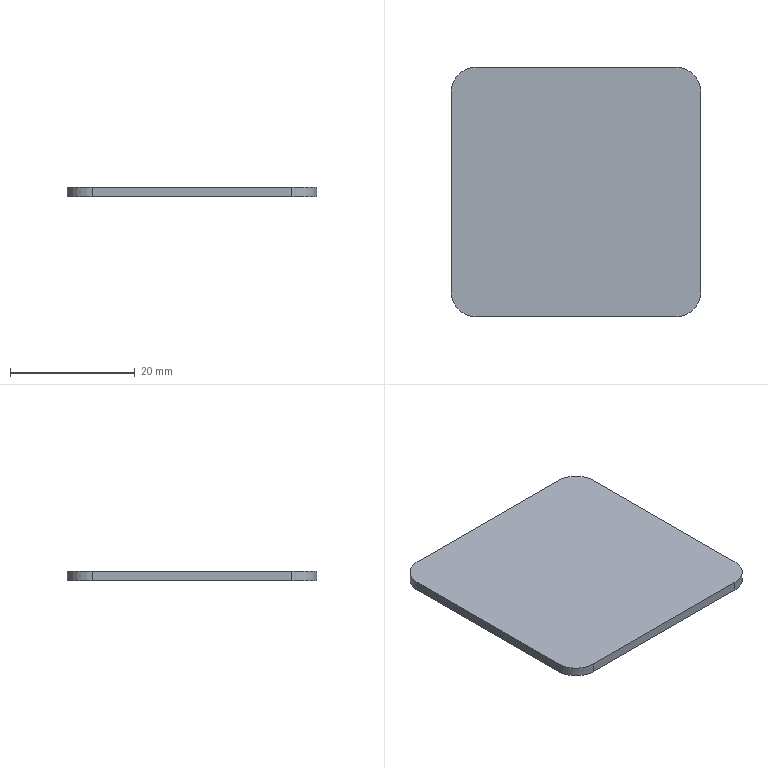Part | SolidWorks | features Extrusion 1 | 1 solid | 10 faces | box 40 x 40 x 1.5 mm | volume 2379 mm3 | plane 6 | cylinder 4 | commonest cylinder face diameters 8 x4
STEP:
#1=CARTESIAN_POINT('',(0.,4.,0.));
#2=VERTEX_POINT('',#1);
#3=CARTESIAN_POINT('',(4.,0.,0.));
#4=VERTEX_POINT('',#3);
#5=CARTESIAN_POINT('',(4.,4.,0.));
#6=DIRECTION('',(0.,0.,1.));
#7=DIRECTION('',(1.,0.,0.));
#8=AXIS2_PLACEMENT_3D('',#5,#6,#7);
#9=CIRCLE('',#8,4.);
#10=EDGE_CURVE('',#2,#4,#9,.T.);
#11=ORIENTED_EDGE('',*,*,#10,.T.);
#12=CARTESIAN_POINT('',(4.,0.,1.5));
#13=VERTEX_POINT('',#12);
#14=CARTESIAN_POINT('',(4.,0.,1.5));
#15=DIRECTION('',(0.,0.,-1.));
#16=VECTOR('',#15,1000.);
#17=LINE('',#14,#16);
#18=EDGE_CURVE('',#13,#4,#17,.T.);
#19=ORIENTED_EDGE('',*,*,#18,.F.);
#20=CARTESIAN_POINT('',(0.,4.,1.5));
#21=VERTEX_POINT('',#20);
#22=CARTESIAN_POINT('',(4.,4.,1.5));
#23=DIRECTION('',(0.,0.,1.));
#24=DIRECTION('',(1.,0.,0.));
#25=AXIS2_PLACEMENT_3D('',#22,#23,#24);
#26=CIRCLE('',#25,4.);
#27=EDGE_CURVE('',#21,#13,#26,.T.);
#28=ORIENTED_EDGE('',*,*,#27,.F.);
#29=CARTESIAN_POINT('',(0.,4.,1.5));
#30=DIRECTION('',(0.,0.,-1.));
#31=VECTOR('',#30,1000.);
#32=LINE('',#29,#31);
#33=EDGE_CURVE('',#21,#2,#32,.T.);
#34=ORIENTED_EDGE('',*,*,#33,.T.);
#35=EDGE_LOOP('',(#11,#19,#28,#34));
#36=FACE_OUTER_BOUND('',#35,.T.);
#37=CARTESIAN_POINT('',(4.,4.,1.5));
#38=DIRECTION('',(0.,0.,-1.));
#39=DIRECTION('',(-1.,0.,0.));
#40=AXIS2_PLACEMENT_3D('',#37,#38,#39);
#41=CYLINDRICAL_SURFACE('',#40,4.);
#42=ADVANCED_FACE('',(#36),#41,.T.);
#43=CARTESIAN_POINT('',(36.,0.,0.));
#44=VERTEX_POINT('',#43);
#45=CARTESIAN_POINT('',(4.,0.,0.));
#46=DIRECTION('',(1.,0.,0.));
#47=VECTOR('',#46,1000.);
#48=LINE('',#45,#47);
#49=EDGE_CURVE('',#4,#44,#48,.T.);
#50=ORIENTED_EDGE('',*,*,#49,.T.);
#51=CARTESIAN_POINT('',(36.,0.,1.5));
#52=VERTEX_POINT('',#51);
#53=CARTESIAN_POINT('',(36.,0.,1.5));
#54=DIRECTION('',(0.,0.,-1.));
#55=VECTOR('',#54,1000.);
#56=LINE('',#53,#55);
#57=EDGE_CURVE('',#52,#44,#56,.T.);
#58=ORIENTED_EDGE('',*,*,#57,.F.);
#59=CARTESIAN_POINT('',(4.,0.,1.5));
#60=DIRECTION('',(1.,0.,0.));
#61=VECTOR('',#60,1000.);
#62=LINE('',#59,#61);
#63=EDGE_CURVE('',#13,#52,#62,.T.);
#64=ORIENTED_EDGE('',*,*,#63,.F.);
#65=ORIENTED_EDGE('',*,*,#18,.T.);
#66=EDGE_LOOP('',(#50,#58,#64,#65));
#67=FACE_OUTER_BOUND('',#66,.T.);
#68=CARTESIAN_POINT('',(4.,0.,1.5));
#69=DIRECTION('',(0.,1.,0.));
#70=DIRECTION('',(0.,0.,1.));
#71=AXIS2_PLACEMENT_3D('',#68,#69,#70);
#72=PLANE('',#71);
#73=ADVANCED_FACE('',(#67),#72,.F.);
#74=CARTESIAN_POINT('',(40.,4.,0.));
#75=VERTEX_POINT('',#74);
#76=CARTESIAN_POINT('',(36.,4.,0.));
#77=DIRECTION('',(0.,0.,1.));
#78=DIRECTION('',(1.,0.,0.));
#79=AXIS2_PLACEMENT_3D('',#76,#77,#78);
#80=CIRCLE('',#79,4.);
#81=EDGE_CURVE('',#44,#75,#80,.T.);
#82=ORIENTED_EDGE('',*,*,#81,.T.);
#83=CARTESIAN_POINT('',(40.,4.,1.5));
#84=VERTEX_POINT('',#83);
#85=CARTESIAN_POINT('',(40.,4.,1.5));
#86=DIRECTION('',(0.,0.,-1.));
#87=VECTOR('',#86,1000.);
#88=LINE('',#85,#87);
#89=EDGE_CURVE('',#84,#75,#88,.T.);
#90=ORIENTED_EDGE('',*,*,#89,.F.);
#91=CARTESIAN_POINT('',(36.,4.,1.5));
#92=DIRECTION('',(0.,0.,1.));
#93=DIRECTION('',(1.,0.,0.));
#94=AXIS2_PLACEMENT_3D('',#91,#92,#93);
#95=CIRCLE('',#94,4.);
#96=EDGE_CURVE('',#52,#84,#95,.T.);
#97=ORIENTED_EDGE('',*,*,#96,.F.);
#98=ORIENTED_EDGE('',*,*,#57,.T.);
#99=EDGE_LOOP('',(#82,#90,#97,#98));
#100=FACE_OUTER_BOUND('',#99,.T.);
#101=CARTESIAN_POINT('',(36.,4.,1.5));
#102=DIRECTION('',(0.,0.,-1.));
#103=DIRECTION('',(-1.,0.,0.));
#104=AXIS2_PLACEMENT_3D('',#101,#102,#103);
#105=CYLINDRICAL_SURFACE('',#104,4.);
#106=ADVANCED_FACE('',(#100),#105,.T.);
#107=CARTESIAN_POINT('',(40.,36.,0.));
#108=VERTEX_POINT('',#107);
#109=CARTESIAN_POINT('',(40.,4.,0.));
#110=DIRECTION('',(0.,1.,0.));
#111=VECTOR('',#110,1000.);
#112=LINE('',#109,#111);
#113=EDGE_CURVE('',#75,#108,#112,.T.);
#114=ORIENTED_EDGE('',*,*,#113,.T.);
#115=CARTESIAN_POINT('',(40.,36.,1.5));
#116=VERTEX_POINT('',#115);
#117=CARTESIAN_POINT('',(40.,36.,1.5));
#118=DIRECTION('',(0.,0.,-1.));
#119=VECTOR('',#118,1000.);
#120=LINE('',#117,#119);
#121=EDGE_CURVE('',#116,#108,#120,.T.);
#122=ORIENTED_EDGE('',*,*,#121,.F.);
#123=CARTESIAN_POINT('',(40.,4.,1.5));
#124=DIRECTION('',(0.,1.,0.));
#125=VECTOR('',#124,1000.);
#126=LINE('',#123,#125);
#127=EDGE_CURVE('',#84,#116,#126,.T.);
#128=ORIENTED_EDGE('',*,*,#127,.F.);
#129=ORIENTED_EDGE('',*,*,#89,.T.);
#130=EDGE_LOOP('',(#114,#122,#128,#129));
#131=FACE_OUTER_BOUND('',#130,.T.);
#132=CARTESIAN_POINT('',(40.,4.,1.5));
#133=DIRECTION('',(-1.,0.,0.));
#134=DIRECTION('',(0.,0.,1.));
#135=AXIS2_PLACEMENT_3D('',#132,#133,#134);
#136=PLANE('',#135);
#137=ADVANCED_FACE('',(#131),#136,.F.);
#138=CARTESIAN_POINT('',(36.,40.,0.));
#139=VERTEX_POINT('',#138);
#140=CARTESIAN_POINT('',(36.,36.,0.));
#141=DIRECTION('',(0.,0.,1.));
#142=DIRECTION('',(1.,0.,0.));
#143=AXIS2_PLACEMENT_3D('',#140,#141,#142);
#144=CIRCLE('',#143,4.);
#145=EDGE_CURVE('',#108,#139,#144,.T.);
#146=ORIENTED_EDGE('',*,*,#145,.T.);
#147=CARTESIAN_POINT('',(36.,40.,1.5));
#148=VERTEX_POINT('',#147);
#149=CARTESIAN_POINT('',(36.,40.,1.5));
#150=DIRECTION('',(0.,0.,-1.));
#151=VECTOR('',#150,1000.);
#152=LINE('',#149,#151);
#153=EDGE_CURVE('',#148,#139,#152,.T.);
#154=ORIENTED_EDGE('',*,*,#153,.F.);
#155=CARTESIAN_POINT('',(36.,36.,1.5));
#156=DIRECTION('',(0.,0.,1.));
#157=DIRECTION('',(1.,0.,0.));
#158=AXIS2_PLACEMENT_3D('',#155,#156,#157);
#159=CIRCLE('',#158,4.);
#160=EDGE_CURVE('',#116,#148,#159,.T.);
#161=ORIENTED_EDGE('',*,*,#160,.F.);
#162=ORIENTED_EDGE('',*,*,#121,.T.);
#163=EDGE_LOOP('',(#146,#154,#161,#162));
#164=FACE_OUTER_BOUND('',#163,.T.);
#165=CARTESIAN_POINT('',(36.,36.,1.5));
#166=DIRECTION('',(0.,0.,-1.));
#167=DIRECTION('',(-1.,0.,0.));
#168=AXIS2_PLACEMENT_3D('',#165,#166,#167);
#169=CYLINDRICAL_SURFACE('',#168,4.);
#170=ADVANCED_FACE('',(#164),#169,.T.);
#171=CARTESIAN_POINT('',(4.,40.,0.));
#172=VERTEX_POINT('',#171);
#173=CARTESIAN_POINT('',(4.,40.,0.));
#174=DIRECTION('',(-1.,0.,0.));
#175=VECTOR('',#174,1000.);
#176=LINE('',#173,#175);
#177=EDGE_CURVE('',#139,#172,#176,.T.);
#178=ORIENTED_EDGE('',*,*,#177,.T.);
#179=CARTESIAN_POINT('',(4.,40.,1.5));
#180=VERTEX_POINT('',#179);
#181=CARTESIAN_POINT('',(4.,40.,1.5));
#182=DIRECTION('',(0.,0.,-1.));
#183=VECTOR('',#182,1000.);
#184=LINE('',#181,#183);
#185=EDGE_CURVE('',#180,#172,#184,.T.);
#186=ORIENTED_EDGE('',*,*,#185,.F.);
#187=CARTESIAN_POINT('',(4.,40.,1.5));
#188=DIRECTION('',(-1.,0.,0.));
#189=VECTOR('',#188,1000.);
#190=LINE('',#187,#189);
#191=EDGE_CURVE('',#148,#180,#190,.T.);
#192=ORIENTED_EDGE('',*,*,#191,.F.);
#193=ORIENTED_EDGE('',*,*,#153,.T.);
#194=EDGE_LOOP('',(#178,#186,#192,#193));
#195=FACE_OUTER_BOUND('',#194,.T.);
#196=CARTESIAN_POINT('',(4.,40.,1.5));
#197=DIRECTION('',(0.,-1.,0.));
#198=DIRECTION('',(0.,0.,-1.));
#199=AXIS2_PLACEMENT_3D('',#196,#197,#198);
#200=PLANE('',#199);
#201=ADVANCED_FACE('',(#195),#200,.F.);
#202=CARTESIAN_POINT('',(0.,36.,0.));
#203=VERTEX_POINT('',#202);
#204=CARTESIAN_POINT('',(4.,36.,0.));
#205=DIRECTION('',(0.,0.,1.));
#206=DIRECTION('',(1.,0.,0.));
#207=AXIS2_PLACEMENT_3D('',#204,#205,#206);
#208=CIRCLE('',#207,4.);
#209=EDGE_CURVE('',#172,#203,#208,.T.);
#210=ORIENTED_EDGE('',*,*,#209,.T.);
#211=CARTESIAN_POINT('',(0.,36.,1.5));
#212=VERTEX_POINT('',#211);
#213=CARTESIAN_POINT('',(0.,36.,1.5));
#214=DIRECTION('',(0.,0.,-1.));
#215=VECTOR('',#214,1000.);
#216=LINE('',#213,#215);
#217=EDGE_CURVE('',#212,#203,#216,.T.);
#218=ORIENTED_EDGE('',*,*,#217,.F.);
#219=CARTESIAN_POINT('',(4.,36.,1.5));
#220=DIRECTION('',(0.,0.,1.));
#221=DIRECTION('',(1.,0.,0.));
#222=AXIS2_PLACEMENT_3D('',#219,#220,#221);
#223=CIRCLE('',#222,4.);
#224=EDGE_CURVE('',#180,#212,#223,.T.);
#225=ORIENTED_EDGE('',*,*,#224,.F.);
#226=ORIENTED_EDGE('',*,*,#185,.T.);
#227=EDGE_LOOP('',(#210,#218,#225,#226));
#228=FACE_OUTER_BOUND('',#227,.T.);
#229=CARTESIAN_POINT('',(4.,36.,1.5));
#230=DIRECTION('',(0.,0.,-1.));
#231=DIRECTION('',(-1.,0.,0.));
#232=AXIS2_PLACEMENT_3D('',#229,#230,#231);
#233=CYLINDRICAL_SURFACE('',#232,4.);
#234=ADVANCED_FACE('',(#228),#233,.T.);
#235=CARTESIAN_POINT('',(0.,4.,0.));
#236=DIRECTION('',(0.,-1.,0.));
#237=VECTOR('',#236,1000.);
#238=LINE('',#235,#237);
#239=EDGE_CURVE('',#203,#2,#238,.T.);
#240=ORIENTED_EDGE('',*,*,#239,.T.);
#241=ORIENTED_EDGE('',*,*,#33,.F.);
#242=CARTESIAN_POINT('',(0.,4.,1.5));
#243=DIRECTION('',(0.,-1.,0.));
#244=VECTOR('',#243,1000.);
#245=LINE('',#242,#244);
#246=EDGE_CURVE('',#212,#21,#245,.T.);
#247=ORIENTED_EDGE('',*,*,#246,.F.);
#248=ORIENTED_EDGE('',*,*,#217,.T.);
#249=EDGE_LOOP('',(#240,#241,#247,#248));
#250=FACE_OUTER_BOUND('',#249,.T.);
#251=CARTESIAN_POINT('',(0.,4.,1.5));
#252=DIRECTION('',(1.,0.,0.));
#253=DIRECTION('',(0.,0.,-1.));
#254=AXIS2_PLACEMENT_3D('',#251,#252,#253);
#255=PLANE('',#254);
#256=ADVANCED_FACE('',(#250),#255,.F.);
#257=ORIENTED_EDGE('',*,*,#27,.T.);
#258=ORIENTED_EDGE('',*,*,#63,.T.);
#259=ORIENTED_EDGE('',*,*,#96,.T.);
#260=ORIENTED_EDGE('',*,*,#127,.T.);
#261=ORIENTED_EDGE('',*,*,#160,.T.);
#262=ORIENTED_EDGE('',*,*,#191,.T.);
#263=ORIENTED_EDGE('',*,*,#224,.T.);
#264=ORIENTED_EDGE('',*,*,#246,.T.);
#265=EDGE_LOOP('',(#257,#258,#259,#260,#261,#262,#263,#264));
#266=FACE_OUTER_BOUND('',#265,.T.);
#267=CARTESIAN_POINT('',(4.,4.,1.5));
#268=DIRECTION('',(0.,0.,1.));
#269=DIRECTION('',(1.,0.,0.));
#270=AXIS2_PLACEMENT_3D('',#267,#268,#269);
#271=PLANE('',#270);
#272=ADVANCED_FACE('',(#266),#271,.T.);
#273=ORIENTED_EDGE('',*,*,#10,.F.);
#274=ORIENTED_EDGE('',*,*,#239,.F.);
#275=ORIENTED_EDGE('',*,*,#209,.F.);
#276=ORIENTED_EDGE('',*,*,#177,.F.);
#277=ORIENTED_EDGE('',*,*,#145,.F.);
#278=ORIENTED_EDGE('',*,*,#113,.F.);
#279=ORIENTED_EDGE('',*,*,#81,.F.);
#280=ORIENTED_EDGE('',*,*,#49,.F.);
#281=EDGE_LOOP('',(#273,#274,#275,#276,#277,#278,#279,#280));
#282=FACE_OUTER_BOUND('',#281,.T.);
#283=CARTESIAN_POINT('',(4.,4.,0.));
#284=DIRECTION('',(0.,0.,1.));
#285=DIRECTION('',(1.,0.,0.));
#286=AXIS2_PLACEMENT_3D('',#283,#284,#285);
#287=PLANE('',#286);
#288=ADVANCED_FACE('',(#282),#287,.F.);
#289=CLOSED_SHELL('',(#42,#73,#106,#137,#170,#201,#234,#256,#272,#288));
#290=MANIFOLD_SOLID_BREP('',#289);
#291=CARTESIAN_POINT('',(0.,0.,0.));
#292=DIRECTION('',(0.,0.,1.));
#293=DIRECTION('',(1.,0.,0.));
#294=AXIS2_PLACEMENT_3D('',#291,#292,#293);
#295=(LENGTH_UNIT()NAMED_UNIT(*)SI_UNIT(.MILLI.,.METRE.));
#296=UNCERTAINTY_MEASURE_WITH_UNIT(LENGTH_MEASURE(0.00001),#295,'','');
#297=(NAMED_UNIT(*)PLANE_ANGLE_UNIT()SI_UNIT($,.RADIAN.));
#298=(NAMED_UNIT(*)SI_UNIT($,.STERADIAN.)SOLID_ANGLE_UNIT());
#299=(GEOMETRIC_REPRESENTATION_CONTEXT(3)GLOBAL_UNCERTAINTY_ASSIGNED_CONTEXT((#296))GLOBAL_UNIT_ASSIGNED_CONTEXT((#295,#297,#298))REPRESENTATION_CONTEXT('',''));
#300=ADVANCED_BREP_SHAPE_REPRESENTATION('',(#290,#294),#299);